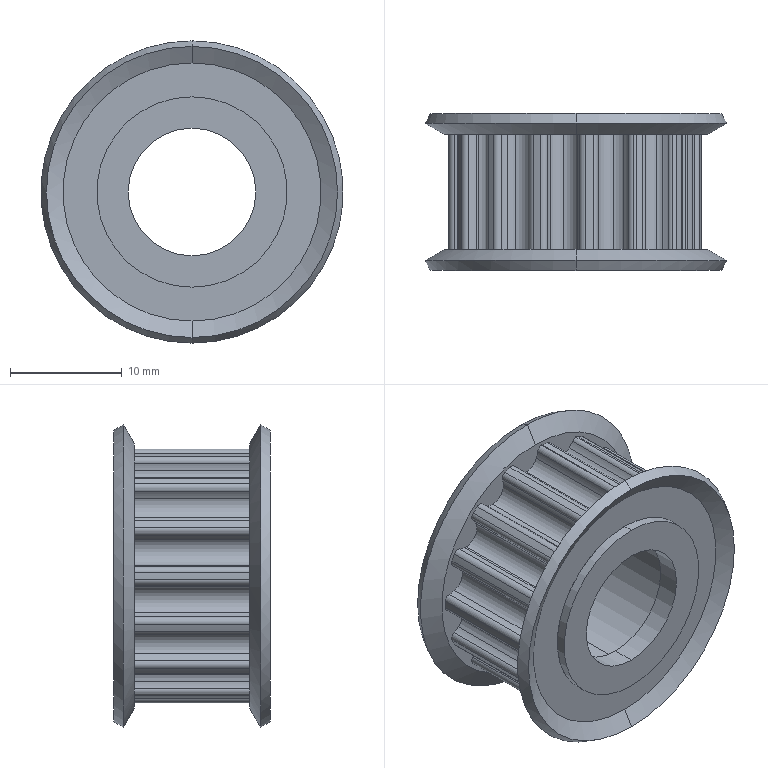Part | NX | features BREP 1 | 1 solid | 147 faces | box 27 x 14 x 27 mm | volume 3178 mm3 | cylinder 120 | cone 16 | plane 11 | commonest cylinder face diameters 1.02 x38 5.08 x31 2.74 x20 22.73 x15 17 x8 13 x4